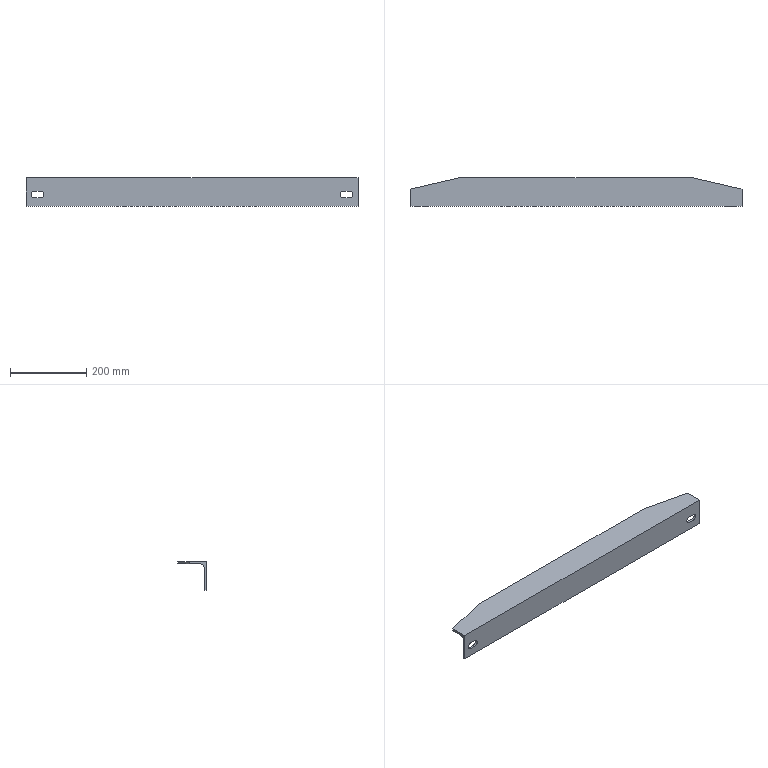Part | SolidWorks | features Chamfer 2, ICE 1, WeldMemberFeat 1, WeldmentFeature 1 | 1 solid | 21 faces | box 871 x 75 x 75 mm | volume 736715 mm3 | plane 14 | cylinder 7 | commonest cylinder face diameters 18 x5 4 x2
STEP:
#1=CARTESIAN_POINT('',(305.5,75.,-4.));
#2=VERTEX_POINT('',#1);
#3=CARTESIAN_POINT('',(-305.5,75.,-4.));
#4=VERTEX_POINT('',#3);
#5=CARTESIAN_POINT('',(435.5,75.,-4.));
#6=DIRECTION('',(-1.,0.,0.));
#7=VECTOR('',#6,1000.);
#8=LINE('',#5,#7);
#9=EDGE_CURVE('',#2,#4,#8,.T.);
#10=ORIENTED_EDGE('',*,*,#9,.T.);
#11=CARTESIAN_POINT('',(-305.5,75.,0.));
#12=VERTEX_POINT('',#11);
#13=CARTESIAN_POINT('',(-305.5,75.,0.));
#14=DIRECTION('',(0.,0.,1.));
#15=VECTOR('',#14,1000.);
#16=LINE('',#13,#15);
#17=EDGE_CURVE('',#4,#12,#16,.T.);
#18=ORIENTED_EDGE('',*,*,#17,.T.);
#19=CARTESIAN_POINT('',(305.5,75.,0.));
#20=VERTEX_POINT('',#19);
#21=CARTESIAN_POINT('',(435.5,75.,0.));
#22=DIRECTION('',(-1.,0.,0.));
#23=VECTOR('',#22,1000.);
#24=LINE('',#21,#23);
#25=EDGE_CURVE('',#20,#12,#24,.T.);
#26=ORIENTED_EDGE('',*,*,#25,.F.);
#27=CARTESIAN_POINT('',(305.5,75.,0.));
#28=DIRECTION('',(0.,0.,-1.));
#29=VECTOR('',#28,1000.);
#30=LINE('',#27,#29);
#31=EDGE_CURVE('',#20,#2,#30,.T.);
#32=ORIENTED_EDGE('',*,*,#31,.T.);
#33=EDGE_LOOP('',(#10,#18,#26,#32));
#34=FACE_OUTER_BOUND('',#33,.T.);
#35=CARTESIAN_POINT('',(435.5,75.,0.));
#36=DIRECTION('',(0.,-1.,0.));
#37=DIRECTION('',(0.,0.,-1.));
#38=AXIS2_PLACEMENT_3D('',#35,#36,#37);
#39=PLANE('',#38);
#40=ADVANCED_FACE('',(#34),#39,.F.);
#41=ORIENTED_EDGE('',*,*,#25,.T.);
#42=CARTESIAN_POINT('',(-435.5,45.,0.));
#43=VERTEX_POINT('',#42);
#44=CARTESIAN_POINT('',(-305.5,75.,0.));
#45=DIRECTION('',(-0.9744,-0.2249,0.));
#46=VECTOR('',#45,1000.);
#47=LINE('',#44,#46);
#48=EDGE_CURVE('',#12,#43,#47,.T.);
#49=ORIENTED_EDGE('',*,*,#48,.T.);
#50=CARTESIAN_POINT('',(-435.5,0.,0.));
#51=VERTEX_POINT('',#50);
#52=CARTESIAN_POINT('',(-435.5,75.,0.));
#53=DIRECTION('',(0.,-1.,0.));
#54=VECTOR('',#53,1000.);
#55=LINE('',#52,#54);
#56=EDGE_CURVE('',#43,#51,#55,.T.);
#57=ORIENTED_EDGE('',*,*,#56,.T.);
#58=CARTESIAN_POINT('',(435.5,0.,0.));
#59=VERTEX_POINT('',#58);
#60=CARTESIAN_POINT('',(435.5,0.,0.));
#61=DIRECTION('',(-1.,0.,0.));
#62=VECTOR('',#61,1000.);
#63=LINE('',#60,#62);
#64=EDGE_CURVE('',#59,#51,#63,.T.);
#65=ORIENTED_EDGE('',*,*,#64,.F.);
#66=CARTESIAN_POINT('',(435.5,45.,0.));
#67=VERTEX_POINT('',#66);
#68=CARTESIAN_POINT('',(435.5,75.,0.));
#69=DIRECTION('',(0.,-1.,0.));
#70=VECTOR('',#69,1000.);
#71=LINE('',#68,#70);
#72=EDGE_CURVE('',#67,#59,#71,.T.);
#73=ORIENTED_EDGE('',*,*,#72,.F.);
#74=CARTESIAN_POINT('',(435.5,45.,0.));
#75=DIRECTION('',(-0.9744,0.2249,0.));
#76=VECTOR('',#75,1000.);
#77=LINE('',#74,#76);
#78=EDGE_CURVE('',#67,#20,#77,.T.);
#79=ORIENTED_EDGE('',*,*,#78,.T.);
#80=EDGE_LOOP('',(#41,#49,#57,#65,#73,#79));
#81=FACE_OUTER_BOUND('',#80,.T.);
#82=CARTESIAN_POINT('',(435.5,75.,0.));
#83=DIRECTION('',(0.,0.,-1.));
#84=DIRECTION('',(0.,1.,0.));
#85=AXIS2_PLACEMENT_3D('',#82,#83,#84);
#86=PLANE('',#85);
#87=ADVANCED_FACE('',(#81),#86,.F.);
#88=CARTESIAN_POINT('',(-413.,0.,-53.));
#89=VERTEX_POINT('',#88);
#90=CARTESIAN_POINT('',(-398.,0.,-53.));
#91=VERTEX_POINT('',#90);
#92=CARTESIAN_POINT('',(-413.,0.,-53.));
#93=DIRECTION('',(1.,0.,0.));
#94=VECTOR('',#93,1000.);
#95=LINE('',#92,#94);
#96=EDGE_CURVE('',#89,#91,#95,.T.);
#97=ORIENTED_EDGE('',*,*,#96,.F.);
#98=CARTESIAN_POINT('',(-413.,0.,-35.));
#99=VERTEX_POINT('',#98);
#100=CARTESIAN_POINT('',(-413.,0.,-44.));
#101=DIRECTION('',(0.,-1.,0.));
#102=DIRECTION('',(0.,0.,1.));
#103=AXIS2_PLACEMENT_3D('',#100,#101,#102);
#104=CIRCLE('',#103,9.);
#105=EDGE_CURVE('',#99,#89,#104,.T.);
#106=ORIENTED_EDGE('',*,*,#105,.F.);
#107=CARTESIAN_POINT('',(-398.,0.,-35.));
#108=VERTEX_POINT('',#107);
#109=CARTESIAN_POINT('',(-413.,0.,-35.));
#110=DIRECTION('',(-1.,0.,0.));
#111=VECTOR('',#110,1000.);
#112=LINE('',#109,#111);
#113=EDGE_CURVE('',#108,#99,#112,.T.);
#114=ORIENTED_EDGE('',*,*,#113,.F.);
#115=CARTESIAN_POINT('',(-398.,0.,-44.));
#116=DIRECTION('',(0.,-1.,0.));
#117=DIRECTION('',(0.,0.,1.));
#118=AXIS2_PLACEMENT_3D('',#115,#116,#117);
#119=CIRCLE('',#118,9.);
#120=EDGE_CURVE('',#91,#108,#119,.T.);
#121=ORIENTED_EDGE('',*,*,#120,.F.);
#122=EDGE_LOOP('',(#97,#106,#114,#121));
#123=FACE_BOUND('',#122,.T.);
#124=CARTESIAN_POINT('',(398.,0.,-53.));
#125=VERTEX_POINT('',#124);
#126=CARTESIAN_POINT('',(413.,0.,-53.));
#127=VERTEX_POINT('',#126);
#128=CARTESIAN_POINT('',(398.,0.,-53.));
#129=DIRECTION('',(1.,0.,0.));
#130=VECTOR('',#129,1000.);
#131=LINE('',#128,#130);
#132=EDGE_CURVE('',#125,#127,#131,.T.);
#133=ORIENTED_EDGE('',*,*,#132,.F.);
#134=CARTESIAN_POINT('',(398.,0.,-35.));
#135=VERTEX_POINT('',#134);
#136=CARTESIAN_POINT('',(398.,0.,-44.));
#137=DIRECTION('',(0.,-1.,0.));
#138=DIRECTION('',(0.,0.,1.));
#139=AXIS2_PLACEMENT_3D('',#136,#137,#138);
#140=CIRCLE('',#139,9.);
#141=EDGE_CURVE('',#135,#125,#140,.T.);
#142=ORIENTED_EDGE('',*,*,#141,.F.);
#143=CARTESIAN_POINT('',(413.,0.,-35.));
#144=VERTEX_POINT('',#143);
#145=CARTESIAN_POINT('',(398.,0.,-35.));
#146=DIRECTION('',(-1.,0.,0.));
#147=VECTOR('',#146,1000.);
#148=LINE('',#145,#147);
#149=EDGE_CURVE('',#144,#135,#148,.T.);
#150=ORIENTED_EDGE('',*,*,#149,.F.);
#151=CARTESIAN_POINT('',(413.,0.,-44.));
#152=DIRECTION('',(0.,-1.,0.));
#153=DIRECTION('',(0.,0.,1.));
#154=AXIS2_PLACEMENT_3D('',#151,#152,#153);
#155=CIRCLE('',#154,9.);
#156=EDGE_CURVE('',#127,#144,#155,.T.);
#157=ORIENTED_EDGE('',*,*,#156,.F.);
#158=EDGE_LOOP('',(#133,#142,#150,#157));
#159=FACE_BOUND('',#158,.T.);
#160=CARTESIAN_POINT('',(-435.5,0.,-75.));
#161=VERTEX_POINT('',#160);
#162=CARTESIAN_POINT('',(-435.5,0.,0.));
#163=DIRECTION('',(0.,0.,-1.));
#164=VECTOR('',#163,1000.);
#165=LINE('',#162,#164);
#166=EDGE_CURVE('',#51,#161,#165,.T.);
#167=ORIENTED_EDGE('',*,*,#166,.T.);
#168=CARTESIAN_POINT('',(435.5,0.,-75.));
#169=VERTEX_POINT('',#168);
#170=CARTESIAN_POINT('',(435.5,0.,-75.));
#171=DIRECTION('',(-1.,0.,0.));
#172=VECTOR('',#171,1000.);
#173=LINE('',#170,#172);
#174=EDGE_CURVE('',#169,#161,#173,.T.);
#175=ORIENTED_EDGE('',*,*,#174,.F.);
#176=CARTESIAN_POINT('',(435.5,0.,0.));
#177=DIRECTION('',(0.,0.,-1.));
#178=VECTOR('',#177,1000.);
#179=LINE('',#176,#178);
#180=EDGE_CURVE('',#59,#169,#179,.T.);
#181=ORIENTED_EDGE('',*,*,#180,.F.);
#182=ORIENTED_EDGE('',*,*,#64,.T.);
#183=EDGE_LOOP('',(#167,#175,#181,#182));
#184=FACE_OUTER_BOUND('',#183,.T.);
#185=CARTESIAN_POINT('',(435.5,0.,0.));
#186=DIRECTION('',(0.,1.,0.));
#187=DIRECTION('',(0.,0.,1.));
#188=AXIS2_PLACEMENT_3D('',#185,#186,#187);
#189=PLANE('',#188);
#190=ADVANCED_FACE('',(#123,#159,#184),#189,.F.);
#191=CARTESIAN_POINT('',(-435.5,4.,-75.));
#192=VERTEX_POINT('',#191);
#193=CARTESIAN_POINT('',(-435.5,0.,-75.));
#194=DIRECTION('',(0.,1.,0.));
#195=VECTOR('',#194,1000.);
#196=LINE('',#193,#195);
#197=EDGE_CURVE('',#161,#192,#196,.T.);
#198=ORIENTED_EDGE('',*,*,#197,.T.);
#199=CARTESIAN_POINT('',(435.5,4.,-75.));
#200=VERTEX_POINT('',#199);
#201=CARTESIAN_POINT('',(435.5,4.,-75.));
#202=DIRECTION('',(-1.,0.,0.));
#203=VECTOR('',#202,1000.);
#204=LINE('',#201,#203);
#205=EDGE_CURVE('',#200,#192,#204,.T.);
#206=ORIENTED_EDGE('',*,*,#205,.F.);
#207=CARTESIAN_POINT('',(435.5,0.,-75.));
#208=DIRECTION('',(0.,1.,0.));
#209=VECTOR('',#208,1000.);
#210=LINE('',#207,#209);
#211=EDGE_CURVE('',#169,#200,#210,.T.);
#212=ORIENTED_EDGE('',*,*,#211,.F.);
#213=ORIENTED_EDGE('',*,*,#174,.T.);
#214=EDGE_LOOP('',(#198,#206,#212,#213));
#215=FACE_OUTER_BOUND('',#214,.T.);
#216=CARTESIAN_POINT('',(435.5,0.,-75.));
#217=DIRECTION('',(0.,0.,1.));
#218=DIRECTION('',(0.,-1.,0.));
#219=AXIS2_PLACEMENT_3D('',#216,#217,#218);
#220=PLANE('',#219);
#221=ADVANCED_FACE('',(#215),#220,.F.);
#222=CARTESIAN_POINT('',(-435.5,6.,-73.));
#223=VERTEX_POINT('',#222);
#224=CARTESIAN_POINT('',(-435.5,4.,-73.));
#225=DIRECTION('',(1.,0.,0.));
#226=DIRECTION('',(0.,0.,-1.));
#227=AXIS2_PLACEMENT_3D('',#224,#225,#226);
#228=CIRCLE('',#227,2.);
#229=EDGE_CURVE('',#192,#223,#228,.T.);
#230=ORIENTED_EDGE('',*,*,#229,.T.);
#231=CARTESIAN_POINT('',(435.5,6.,-73.));
#232=VERTEX_POINT('',#231);
#233=CARTESIAN_POINT('',(435.5,6.,-73.));
#234=DIRECTION('',(-1.,0.,0.));
#235=VECTOR('',#234,1000.);
#236=LINE('',#233,#235);
#237=EDGE_CURVE('',#232,#223,#236,.T.);
#238=ORIENTED_EDGE('',*,*,#237,.F.);
#239=CARTESIAN_POINT('',(435.5,4.,-73.));
#240=DIRECTION('',(1.,0.,0.));
#241=DIRECTION('',(0.,0.,-1.));
#242=AXIS2_PLACEMENT_3D('',#239,#240,#241);
#243=CIRCLE('',#242,2.);
#244=EDGE_CURVE('',#200,#232,#243,.T.);
#245=ORIENTED_EDGE('',*,*,#244,.F.);
#246=ORIENTED_EDGE('',*,*,#205,.T.);
#247=EDGE_LOOP('',(#230,#238,#245,#246));
#248=FACE_OUTER_BOUND('',#247,.T.);
#249=CARTESIAN_POINT('',(435.5,4.,-73.));
#250=DIRECTION('',(-1.,0.,0.));
#251=DIRECTION('',(0.,0.,1.));
#252=AXIS2_PLACEMENT_3D('',#249,#250,#251);
#253=CYLINDRICAL_SURFACE('',#252,2.);
#254=ADVANCED_FACE('',(#248),#253,.T.);
#255=CARTESIAN_POINT('',(-413.,6.,-35.));
#256=VERTEX_POINT('',#255);
#257=CARTESIAN_POINT('',(-398.,6.,-35.));
#258=VERTEX_POINT('',#257);
#259=CARTESIAN_POINT('',(-413.,6.,-35.));
#260=DIRECTION('',(1.,0.,0.));
#261=VECTOR('',#260,1000.);
#262=LINE('',#259,#261);
#263=EDGE_CURVE('',#256,#258,#262,.T.);
#264=ORIENTED_EDGE('',*,*,#263,.F.);
#265=CARTESIAN_POINT('',(-413.,6.,-53.));
#266=VERTEX_POINT('',#265);
#267=CARTESIAN_POINT('',(-413.,6.,-44.));
#268=DIRECTION('',(0.,1.,0.));
#269=DIRECTION('',(0.,0.,1.));
#270=AXIS2_PLACEMENT_3D('',#267,#268,#269);
#271=CIRCLE('',#270,9.);
#272=EDGE_CURVE('',#266,#256,#271,.T.);
#273=ORIENTED_EDGE('',*,*,#272,.F.);
#274=CARTESIAN_POINT('',(-398.,6.,-53.));
#275=VERTEX_POINT('',#274);
#276=CARTESIAN_POINT('',(-413.,6.,-53.));
#277=DIRECTION('',(-1.,0.,0.));
#278=VECTOR('',#277,1000.);
#279=LINE('',#276,#278);
#280=EDGE_CURVE('',#275,#266,#279,.T.);
#281=ORIENTED_EDGE('',*,*,#280,.F.);
#282=CARTESIAN_POINT('',(-398.,6.,-44.));
#283=DIRECTION('',(0.,1.,0.));
#284=DIRECTION('',(0.,0.,1.));
#285=AXIS2_PLACEMENT_3D('',#282,#283,#284);
#286=CIRCLE('',#285,9.);
#287=EDGE_CURVE('',#258,#275,#286,.T.);
#288=ORIENTED_EDGE('',*,*,#287,.F.);
#289=EDGE_LOOP('',(#264,#273,#281,#288));
#290=FACE_BOUND('',#289,.T.);
#291=CARTESIAN_POINT('',(398.,6.,-35.));
#292=VERTEX_POINT('',#291);
#293=CARTESIAN_POINT('',(413.,6.,-35.));
#294=VERTEX_POINT('',#293);
#295=CARTESIAN_POINT('',(398.,6.,-35.));
#296=DIRECTION('',(1.,0.,0.));
#297=VECTOR('',#296,1000.);
#298=LINE('',#295,#297);
#299=EDGE_CURVE('',#292,#294,#298,.T.);
#300=ORIENTED_EDGE('',*,*,#299,.F.);
#301=CARTESIAN_POINT('',(398.,6.,-53.));
#302=VERTEX_POINT('',#301);
#303=CARTESIAN_POINT('',(398.,6.,-44.));
#304=DIRECTION('',(0.,1.,0.));
#305=DIRECTION('',(0.,0.,1.));
#306=AXIS2_PLACEMENT_3D('',#303,#304,#305);
#307=CIRCLE('',#306,9.);
#308=EDGE_CURVE('',#302,#292,#307,.T.);
#309=ORIENTED_EDGE('',*,*,#308,.F.);
#310=CARTESIAN_POINT('',(413.,6.,-53.));
#311=VERTEX_POINT('',#310);
#312=CARTESIAN_POINT('',(398.,6.,-53.));
#313=DIRECTION('',(-1.,0.,0.));
#314=VECTOR('',#313,1000.);
#315=LINE('',#312,#314);
#316=EDGE_CURVE('',#311,#302,#315,.T.);
#317=ORIENTED_EDGE('',*,*,#316,.F.);
#318=CARTESIAN_POINT('',(413.,6.,-44.));
#319=DIRECTION('',(0.,1.,0.));
#320=DIRECTION('',(0.,0.,1.));
#321=AXIS2_PLACEMENT_3D('',#318,#319,#320);
#322=CIRCLE('',#321,9.);
#323=EDGE_CURVE('',#294,#311,#322,.T.);
#324=ORIENTED_EDGE('',*,*,#323,.F.);
#325=EDGE_LOOP('',(#300,#309,#317,#324));
#326=FACE_BOUND('',#325,.T.);
#327=CARTESIAN_POINT('',(-435.5,6.,-15.));
#328=VERTEX_POINT('',#327);
#329=CARTESIAN_POINT('',(-435.5,6.,-15.));
#330=DIRECTION('',(0.,0.,1.));
#331=VECTOR('',#330,1000.);
#332=LINE('',#329,#331);
#333=EDGE_CURVE('',#223,#328,#332,.T.);
#334=ORIENTED_EDGE('',*,*,#333,.T.);
#335=CARTESIAN_POINT('',(435.5,6.,-15.));
#336=VERTEX_POINT('',#335);
#337=CARTESIAN_POINT('',(435.5,6.,-15.));
#338=DIRECTION('',(-1.,0.,0.));
#339=VECTOR('',#338,1000.);
#340=LINE('',#337,#339);
#341=EDGE_CURVE('',#336,#328,#340,.T.);
#342=ORIENTED_EDGE('',*,*,#341,.F.);
#343=CARTESIAN_POINT('',(435.5,6.,-15.));
#344=DIRECTION('',(0.,0.,1.));
#345=VECTOR('',#344,1000.);
#346=LINE('',#343,#345);
#347=EDGE_CURVE('',#232,#336,#346,.T.);
#348=ORIENTED_EDGE('',*,*,#347,.F.);
#349=ORIENTED_EDGE('',*,*,#237,.T.);
#350=EDGE_LOOP('',(#334,#342,#348,#349));
#351=FACE_OUTER_BOUND('',#350,.T.);
#352=CARTESIAN_POINT('',(435.5,6.,-15.));
#353=DIRECTION('',(0.,-1.,0.));
#354=DIRECTION('',(0.,0.,-1.));
#355=AXIS2_PLACEMENT_3D('',#352,#353,#354);
#356=PLANE('',#355);
#357=ADVANCED_FACE('',(#290,#326,#351),#356,.F.);
#358=CARTESIAN_POINT('',(-435.5,15.,-6.));
#359=VERTEX_POINT('',#358);
#360=CARTESIAN_POINT('',(-435.5,15.,-15.));
#361=DIRECTION('',(-1.,0.,0.));
#362=DIRECTION('',(0.,0.,-1.));
#363=AXIS2_PLACEMENT_3D('',#360,#361,#362);
#364=CIRCLE('',#363,9.);
#365=EDGE_CURVE('',#328,#359,#364,.T.);
#366=ORIENTED_EDGE('',*,*,#365,.T.);
#367=CARTESIAN_POINT('',(435.5,15.,-6.));
#368=VERTEX_POINT('',#367);
#369=CARTESIAN_POINT('',(435.5,15.,-6.));
#370=DIRECTION('',(-1.,0.,0.));
#371=VECTOR('',#370,1000.);
#372=LINE('',#369,#371);
#373=EDGE_CURVE('',#368,#359,#372,.T.);
#374=ORIENTED_EDGE('',*,*,#373,.F.);
#375=CARTESIAN_POINT('',(435.5,15.,-15.));
#376=DIRECTION('',(-1.,0.,0.));
#377=DIRECTION('',(0.,0.,-1.));
#378=AXIS2_PLACEMENT_3D('',#375,#376,#377);
#379=CIRCLE('',#378,9.);
#380=EDGE_CURVE('',#336,#368,#379,.T.);
#381=ORIENTED_EDGE('',*,*,#380,.F.);
#382=ORIENTED_EDGE('',*,*,#341,.T.);
#383=EDGE_LOOP('',(#366,#374,#381,#382));
#384=FACE_OUTER_BOUND('',#383,.T.);
#385=CARTESIAN_POINT('',(435.5,15.,-15.));
#386=DIRECTION('',(-1.,0.,0.));
#387=DIRECTION('',(0.,0.,1.));
#388=AXIS2_PLACEMENT_3D('',#385,#386,#387);
#389=CYLINDRICAL_SURFACE('',#388,9.);
#390=ADVANCED_FACE('',(#384),#389,.F.);
#391=CARTESIAN_POINT('',(-435.5,45.,-6.));
#392=VERTEX_POINT('',#391);
#393=CARTESIAN_POINT('',(-435.5,73.,-6.));
#394=DIRECTION('',(0.,1.,0.));
#395=VECTOR('',#394,1000.);
#396=LINE('',#393,#395);
#397=EDGE_CURVE('',#359,#392,#396,.T.);
#398=ORIENTED_EDGE('',*,*,#397,.T.);
#399=CARTESIAN_POINT('',(-314.167,73.,-6.));
#400=VERTEX_POINT('',#399);
#401=CARTESIAN_POINT('',(-305.5,75.,-6.));
#402=DIRECTION('',(0.9744,0.2249,0.));
#403=VECTOR('',#402,1000.);
#404=LINE('',#401,#403);
#405=EDGE_CURVE('',#392,#400,#404,.T.);
#406=ORIENTED_EDGE('',*,*,#405,.T.);
#407=CARTESIAN_POINT('',(314.167,73.,-6.));
#408=VERTEX_POINT('',#407);
#409=CARTESIAN_POINT('',(435.5,73.,-6.));
#410=DIRECTION('',(-1.,0.,0.));
#411=VECTOR('',#410,1000.);
#412=LINE('',#409,#411);
#413=EDGE_CURVE('',#408,#400,#412,.T.);
#414=ORIENTED_EDGE('',*,*,#413,.F.);
#415=CARTESIAN_POINT('',(435.5,45.,-6.));
#416=VERTEX_POINT('',#415);
#417=CARTESIAN_POINT('',(435.5,45.,-6.));
#418=DIRECTION('',(0.9744,-0.2249,0.));
#419=VECTOR('',#418,1000.);
#420=LINE('',#417,#419);
#421=EDGE_CURVE('',#408,#416,#420,.T.);
#422=ORIENTED_EDGE('',*,*,#421,.T.);
#423=CARTESIAN_POINT('',(435.5,73.,-6.));
#424=DIRECTION('',(0.,1.,0.));
#425=VECTOR('',#424,1000.);
#426=LINE('',#423,#425);
#427=EDGE_CURVE('',#368,#416,#426,.T.);
#428=ORIENTED_EDGE('',*,*,#427,.F.);
#429=ORIENTED_EDGE('',*,*,#373,.T.);
#430=EDGE_LOOP('',(#398,#406,#414,#422,#428,#429));
#431=FACE_OUTER_BOUND('',#430,.T.);
#432=CARTESIAN_POINT('',(435.5,73.,-6.));
#433=DIRECTION('',(0.,0.,1.));
#434=DIRECTION('',(0.,-1.,0.));
#435=AXIS2_PLACEMENT_3D('',#432,#433,#434);
#436=PLANE('',#435);
#437=ADVANCED_FACE('',(#431),#436,.F.);
#438=ORIENTED_EDGE('',*,*,#413,.T.);
#439=CARTESIAN_POINT('',(-314.167,73.,-6.));
#440=CARTESIAN_POINT('',(-309.09,74.172,-6.));
#441=CARTESIAN_POINT('',(-305.5,75.,-5.172));
#442=CARTESIAN_POINT('',(-305.5,75.,-4.));
#443=(BOUNDED_CURVE()B_SPLINE_CURVE(3,(#439,#440,#441,#442),.UNSPECIFIED.,.F.,.F.)B_SPLINE_CURVE_WITH_KNOTS((4,4),(1.571,3.142),.UNSPECIFIED.)CURVE()GEOMETRIC_REPRESENTATION_ITEM()RATIONAL_B_SPLINE_CURVE((1.,0.8047,0.8047,1.))REPRESENTATION_ITEM(''));
#444=EDGE_CURVE('',#400,#4,#443,.T.);
#445=ORIENTED_EDGE('',*,*,#444,.T.);
#446=ORIENTED_EDGE('',*,*,#9,.F.);
#447=CARTESIAN_POINT('',(305.5,75.,-4.));
#448=CARTESIAN_POINT('',(305.5,75.,-5.172));
#449=CARTESIAN_POINT('',(309.09,74.172,-6.));
#450=CARTESIAN_POINT('',(314.167,73.,-6.));
#451=(BOUNDED_CURVE()B_SPLINE_CURVE(3,(#447,#448,#449,#450),.UNSPECIFIED.,.F.,.F.)B_SPLINE_CURVE_WITH_KNOTS((4,4),(0.,1.571),.UNSPECIFIED.)CURVE()GEOMETRIC_REPRESENTATION_ITEM()RATIONAL_B_SPLINE_CURVE((1.,0.8047,0.8047,1.))REPRESENTATION_ITEM(''));
#452=EDGE_CURVE('',#2,#408,#451,.T.);
#453=ORIENTED_EDGE('',*,*,#452,.T.);
#454=EDGE_LOOP('',(#438,#445,#446,#453));
#455=FACE_OUTER_BOUND('',#454,.T.);
#456=CARTESIAN_POINT('',(435.5,73.,-4.));
#457=DIRECTION('',(-1.,0.,0.));
#458=DIRECTION('',(0.,0.,1.));
#459=AXIS2_PLACEMENT_3D('',#456,#457,#458);
#460=CYLINDRICAL_SURFACE('',#459,2.);
#461=ADVANCED_FACE('',(#455),#460,.T.);
#462=ORIENTED_EDGE('',*,*,#427,.T.);
#463=CARTESIAN_POINT('',(435.5,45.,-4.));
#464=DIRECTION('',(0.,0.,1.));
#465=VECTOR('',#464,1000.);
#466=LINE('',#463,#465);
#467=EDGE_CURVE('',#416,#67,#466,.T.);
#468=ORIENTED_EDGE('',*,*,#467,.T.);
#469=ORIENTED_EDGE('',*,*,#72,.T.);
#470=ORIENTED_EDGE('',*,*,#180,.T.);
#471=ORIENTED_EDGE('',*,*,#211,.T.);
#472=ORIENTED_EDGE('',*,*,#244,.T.);
#473=ORIENTED_EDGE('',*,*,#347,.T.);
#474=ORIENTED_EDGE('',*,*,#380,.T.);
#475=EDGE_LOOP('',(#462,#468,#469,#470,#471,#472,#473,#474));
#476=FACE_OUTER_BOUND('',#475,.T.);
#477=CARTESIAN_POINT('',(435.5,73.,-4.));
#478=DIRECTION('',(-1.,0.,0.));
#479=DIRECTION('',(0.,0.,1.));
#480=AXIS2_PLACEMENT_3D('',#477,#478,#479);
#481=PLANE('',#480);
#482=ADVANCED_FACE('',(#476),#481,.F.);
#483=ORIENTED_EDGE('',*,*,#56,.F.);
#484=CARTESIAN_POINT('',(-435.5,45.,-4.));
#485=DIRECTION('',(0.,0.,-1.));
#486=VECTOR('',#485,1000.);
#487=LINE('',#484,#486);
#488=EDGE_CURVE('',#43,#392,#487,.T.);
#489=ORIENTED_EDGE('',*,*,#488,.T.);
#490=ORIENTED_EDGE('',*,*,#397,.F.);
#491=ORIENTED_EDGE('',*,*,#365,.F.);
#492=ORIENTED_EDGE('',*,*,#333,.F.);
#493=ORIENTED_EDGE('',*,*,#229,.F.);
#494=ORIENTED_EDGE('',*,*,#197,.F.);
#495=ORIENTED_EDGE('',*,*,#166,.F.);
#496=EDGE_LOOP('',(#483,#489,#490,#491,#492,#493,#494,#495));
#497=FACE_OUTER_BOUND('',#496,.T.);
#498=CARTESIAN_POINT('',(-435.5,73.,-4.));
#499=DIRECTION('',(-1.,0.,0.));
#500=DIRECTION('',(0.,0.,1.));
#501=AXIS2_PLACEMENT_3D('',#498,#499,#500);
#502=PLANE('',#501);
#503=ADVANCED_FACE('',(#497),#502,.T.);
#504=ORIENTED_EDGE('',*,*,#141,.T.);
#505=CARTESIAN_POINT('',(398.,-0.001,-53.));
#506=DIRECTION('',(0.,1.,0.));
#507=VECTOR('',#506,1000.);
#508=LINE('',#505,#507);
#509=EDGE_CURVE('',#125,#302,#508,.T.);
#510=ORIENTED_EDGE('',*,*,#509,.T.);
#511=ORIENTED_EDGE('',*,*,#308,.T.);
#512=CARTESIAN_POINT('',(398.,-0.001,-35.));
#513=DIRECTION('',(0.,1.,0.));
#514=VECTOR('',#513,1000.);
#515=LINE('',#512,#514);
#516=EDGE_CURVE('',#135,#292,#515,.T.);
#517=ORIENTED_EDGE('',*,*,#516,.F.);
#518=EDGE_LOOP('',(#504,#510,#511,#517));
#519=FACE_OUTER_BOUND('',#518,.T.);
#520=CARTESIAN_POINT('',(398.,-0.001,-44.));
#521=DIRECTION('',(0.,1.,0.));
#522=DIRECTION('',(0.,0.,1.));
#523=AXIS2_PLACEMENT_3D('',#520,#521,#522);
#524=CYLINDRICAL_SURFACE('',#523,9.);
#525=ADVANCED_FACE('',(#519),#524,.F.);
#526=ORIENTED_EDGE('',*,*,#132,.T.);
#527=CARTESIAN_POINT('',(413.,-0.001,-53.));
#528=DIRECTION('',(0.,1.,0.));
#529=VECTOR('',#528,1000.);
#530=LINE('',#527,#529);
#531=EDGE_CURVE('',#127,#311,#530,.T.);
#532=ORIENTED_EDGE('',*,*,#531,.T.);
#533=ORIENTED_EDGE('',*,*,#316,.T.);
#534=ORIENTED_EDGE('',*,*,#509,.F.);
#535=EDGE_LOOP('',(#526,#532,#533,#534));
#536=FACE_OUTER_BOUND('',#535,.T.);
#537=CARTESIAN_POINT('',(398.,-0.001,-53.));
#538=DIRECTION('',(0.,0.,-1.));
#539=DIRECTION('',(0.,1.,0.));
#540=AXIS2_PLACEMENT_3D('',#537,#538,#539);
#541=PLANE('',#540);
#542=ADVANCED_FACE('',(#536),#541,.F.);
#543=ORIENTED_EDGE('',*,*,#156,.T.);
#544=CARTESIAN_POINT('',(413.,-0.001,-35.));
#545=DIRECTION('',(0.,1.,0.));
#546=VECTOR('',#545,1000.);
#547=LINE('',#544,#546);
#548=EDGE_CURVE('',#144,#294,#547,.T.);
#549=ORIENTED_EDGE('',*,*,#548,.T.);
#550=ORIENTED_EDGE('',*,*,#323,.T.);
#551=ORIENTED_EDGE('',*,*,#531,.F.);
#552=EDGE_LOOP('',(#543,#549,#550,#551));
#553=FACE_OUTER_BOUND('',#552,.T.);
#554=CARTESIAN_POINT('',(413.,-0.001,-44.));
#555=DIRECTION('',(0.,1.,0.));
#556=DIRECTION('',(0.,0.,1.));
#557=AXIS2_PLACEMENT_3D('',#554,#555,#556);
#558=CYLINDRICAL_SURFACE('',#557,9.);
#559=ADVANCED_FACE('',(#553),#558,.F.);
#560=ORIENTED_EDGE('',*,*,#149,.T.);
#561=ORIENTED_EDGE('',*,*,#516,.T.);
#562=ORIENTED_EDGE('',*,*,#299,.T.);
#563=ORIENTED_EDGE('',*,*,#548,.F.);
#564=EDGE_LOOP('',(#560,#561,#562,#563));
#565=FACE_OUTER_BOUND('',#564,.T.);
#566=CARTESIAN_POINT('',(398.,-0.001,-35.));
#567=DIRECTION('',(0.,0.,1.));
#568=DIRECTION('',(1.,0.,0.));
#569=AXIS2_PLACEMENT_3D('',#566,#567,#568);
#570=PLANE('',#569);
#571=ADVANCED_FACE('',(#565),#570,.F.);
#572=ORIENTED_EDGE('',*,*,#105,.T.);
#573=CARTESIAN_POINT('',(-413.,-0.001,-53.));
#574=DIRECTION('',(0.,1.,0.));
#575=VECTOR('',#574,1000.);
#576=LINE('',#573,#575);
#577=EDGE_CURVE('',#89,#266,#576,.T.);
#578=ORIENTED_EDGE('',*,*,#577,.T.);
#579=ORIENTED_EDGE('',*,*,#272,.T.);
#580=CARTESIAN_POINT('',(-413.,-0.001,-35.));
#581=DIRECTION('',(0.,1.,0.));
#582=VECTOR('',#581,1000.);
#583=LINE('',#580,#582);
#584=EDGE_CURVE('',#99,#256,#583,.T.);
#585=ORIENTED_EDGE('',*,*,#584,.F.);
#586=EDGE_LOOP('',(#572,#578,#579,#585));
#587=FACE_OUTER_BOUND('',#586,.T.);
#588=CARTESIAN_POINT('',(-413.,-0.001,-44.));
#589=DIRECTION('',(0.,1.,0.));
#590=DIRECTION('',(0.,0.,1.));
#591=AXIS2_PLACEMENT_3D('',#588,#589,#590);
#592=CYLINDRICAL_SURFACE('',#591,9.);
#593=ADVANCED_FACE('',(#587),#592,.F.);
#594=ORIENTED_EDGE('',*,*,#96,.T.);
#595=CARTESIAN_POINT('',(-398.,-0.001,-53.));
#596=DIRECTION('',(0.,1.,0.));
#597=VECTOR('',#596,1000.);
#598=LINE('',#595,#597);
#599=EDGE_CURVE('',#91,#275,#598,.T.);
#600=ORIENTED_EDGE('',*,*,#599,.T.);
#601=ORIENTED_EDGE('',*,*,#280,.T.);
#602=ORIENTED_EDGE('',*,*,#577,.F.);
#603=EDGE_LOOP('',(#594,#600,#601,#602));
#604=FACE_OUTER_BOUND('',#603,.T.);
#605=CARTESIAN_POINT('',(-413.,-0.001,-53.));
#606=DIRECTION('',(0.,0.,-1.));
#607=DIRECTION('',(0.,1.,0.));
#608=AXIS2_PLACEMENT_3D('',#605,#606,#607);
#609=PLANE('',#608);
#610=ADVANCED_FACE('',(#604),#609,.F.);
#611=ORIENTED_EDGE('',*,*,#120,.T.);
#612=CARTESIAN_POINT('',(-398.,-0.001,-35.));
#613=DIRECTION('',(0.,1.,0.));
#614=VECTOR('',#613,1000.);
#615=LINE('',#612,#614);
#616=EDGE_CURVE('',#108,#258,#615,.T.);
#617=ORIENTED_EDGE('',*,*,#616,.T.);
#618=ORIENTED_EDGE('',*,*,#287,.T.);
#619=ORIENTED_EDGE('',*,*,#599,.F.);
#620=EDGE_LOOP('',(#611,#617,#618,#619));
#621=FACE_OUTER_BOUND('',#620,.T.);
#622=CARTESIAN_POINT('',(-398.,-0.001,-44.));
#623=DIRECTION('',(0.,1.,0.));
#624=DIRECTION('',(0.,0.,1.));
#625=AXIS2_PLACEMENT_3D('',#622,#623,#624);
#626=CYLINDRICAL_SURFACE('',#625,9.);
#627=ADVANCED_FACE('',(#621),#626,.F.);
#628=ORIENTED_EDGE('',*,*,#113,.T.);
#629=ORIENTED_EDGE('',*,*,#584,.T.);
#630=ORIENTED_EDGE('',*,*,#263,.T.);
#631=ORIENTED_EDGE('',*,*,#616,.F.);
#632=EDGE_LOOP('',(#628,#629,#630,#631));
#633=FACE_OUTER_BOUND('',#632,.T.);
#634=CARTESIAN_POINT('',(-413.,-0.001,-35.));
#635=DIRECTION('',(0.,0.,1.));
#636=DIRECTION('',(1.,0.,0.));
#637=AXIS2_PLACEMENT_3D('',#634,#635,#636);
#638=PLANE('',#637);
#639=ADVANCED_FACE('',(#633),#638,.F.);
#640=ORIENTED_EDGE('',*,*,#452,.F.);
#641=ORIENTED_EDGE('',*,*,#31,.F.);
#642=ORIENTED_EDGE('',*,*,#78,.F.);
#643=ORIENTED_EDGE('',*,*,#467,.F.);
#644=ORIENTED_EDGE('',*,*,#421,.F.);
#645=EDGE_LOOP('',(#640,#641,#642,#643,#644));
#646=FACE_OUTER_BOUND('',#645,.T.);
#647=CARTESIAN_POINT('',(435.5,45.,-4.));
#648=DIRECTION('',(-0.2249,-0.9744,0.));
#649=DIRECTION('',(0.,0.,1.));
#650=AXIS2_PLACEMENT_3D('',#647,#648,#649);
#651=PLANE('',#650);
#652=ADVANCED_FACE('',(#646),#651,.F.);
#653=ORIENTED_EDGE('',*,*,#405,.F.);
#654=ORIENTED_EDGE('',*,*,#488,.F.);
#655=ORIENTED_EDGE('',*,*,#48,.F.);
#656=ORIENTED_EDGE('',*,*,#17,.F.);
#657=ORIENTED_EDGE('',*,*,#444,.F.);
#658=EDGE_LOOP('',(#653,#654,#655,#656,#657));
#659=FACE_OUTER_BOUND('',#658,.T.);
#660=CARTESIAN_POINT('',(-305.5,75.,0.));
#661=DIRECTION('',(-0.2249,0.9744,0.));
#662=DIRECTION('',(0.,0.,-1.));
#663=AXIS2_PLACEMENT_3D('',#660,#661,#662);
#664=PLANE('',#663);
#665=ADVANCED_FACE('',(#659),#664,.T.);
#666=CLOSED_SHELL('',(#40,#87,#190,#221,#254,#357,#390,#437,#461,#482,#503,#525,#542,#559,#571,#593,#610,#627,#639,#652,#665));
#667=MANIFOLD_SOLID_BREP('',#666);
#668=CARTESIAN_POINT('',(0.,0.,0.));
#669=DIRECTION('',(0.,0.,1.));
#670=DIRECTION('',(1.,0.,0.));
#671=AXIS2_PLACEMENT_3D('',#668,#669,#670);
#672=(LENGTH_UNIT()NAMED_UNIT(*)SI_UNIT(.MILLI.,.METRE.));
#673=UNCERTAINTY_MEASURE_WITH_UNIT(LENGTH_MEASURE(0.00001),#672,'','');
#674=(NAMED_UNIT(*)PLANE_ANGLE_UNIT()SI_UNIT($,.RADIAN.));
#675=(NAMED_UNIT(*)SI_UNIT($,.STERADIAN.)SOLID_ANGLE_UNIT());
#676=(GEOMETRIC_REPRESENTATION_CONTEXT(3)GLOBAL_UNCERTAINTY_ASSIGNED_CONTEXT((#673))GLOBAL_UNIT_ASSIGNED_CONTEXT((#672,#674,#675))REPRESENTATION_CONTEXT('',''));
#677=ADVANCED_BREP_SHAPE_REPRESENTATION('',(#667,#671),#676);